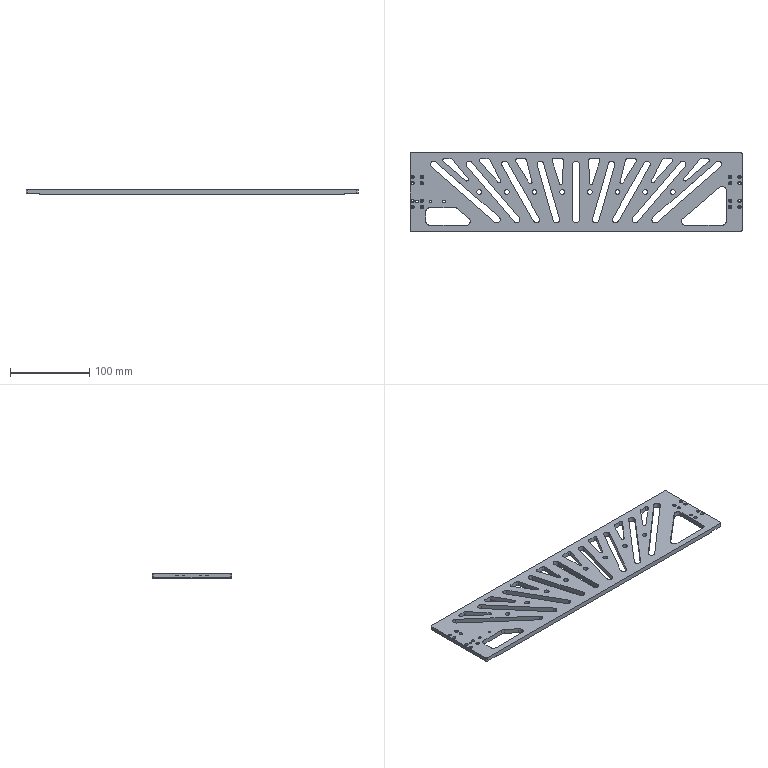Part | STEP file | PN_0002 | 1 solid | 231 faces | box 420 x 100 x 6 mm | volume 175315 mm3 | cylinder 156 | plane 75 | commonest cylinder face diameters 2.4 x32 4 x32 4.3 x32 8.1 x26 6 x16 10 x8